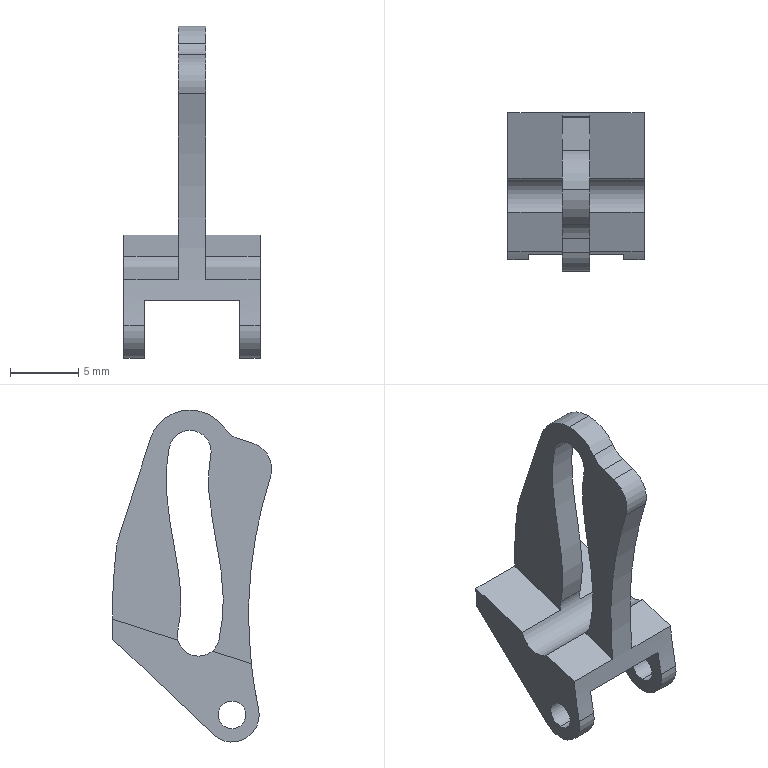Part | SolidWorks | features ICE 2, Extrusion 1, Fillet 1 | 1 solid | 33 faces | box 10 x 11.684 x 24.374 mm | volume 433.075 mm3 | cylinder 16 | plane 15 | spline 2 | commonest cylinder face diameters 4 x5 2.02 x4 3.1 x3 6.1 x2 66 x1 86 x1
STEP:
#1=CARTESIAN_POINT('',(5.,10.718,-6.14));
#2=VERTEX_POINT('',#1);
#3=CARTESIAN_POINT('',(5.,10.718,-8.16));
#4=VERTEX_POINT('',#3);
#5=CARTESIAN_POINT('',(5.,10.718,-7.15));
#6=DIRECTION('',(1.,0.,0.));
#7=DIRECTION('',(0.,0.,-1.));
#8=AXIS2_PLACEMENT_3D('',#5,#6,#7);
#9=CIRCLE('',#8,1.01);
#10=EDGE_CURVE('',#2,#4,#9,.T.);
#11=ORIENTED_EDGE('',*,*,#10,.T.);
#12=CARTESIAN_POINT('',(3.5,10.718,-8.16));
#13=VERTEX_POINT('',#12);
#14=CARTESIAN_POINT('',(1.,10.718,-8.16));
#15=DIRECTION('',(-1.,0.,0.));
#16=VECTOR('',#15,1000.);
#17=LINE('',#14,#16);
#18=EDGE_CURVE('',#4,#13,#17,.T.);
#19=ORIENTED_EDGE('',*,*,#18,.T.);
#20=CARTESIAN_POINT('',(3.5,10.718,-6.14));
#21=VERTEX_POINT('',#20);
#22=CARTESIAN_POINT('',(3.5,10.718,-7.15));
#23=DIRECTION('',(1.,0.,0.));
#24=DIRECTION('',(0.,0.,-1.));
#25=AXIS2_PLACEMENT_3D('',#22,#23,#24);
#26=CIRCLE('',#25,1.01);
#27=EDGE_CURVE('',#21,#13,#26,.T.);
#28=ORIENTED_EDGE('',*,*,#27,.F.);
#29=CARTESIAN_POINT('',(1.,10.718,-6.14));
#30=DIRECTION('',(-1.,0.,0.));
#31=VECTOR('',#30,1000.);
#32=LINE('',#29,#31);
#33=EDGE_CURVE('',#2,#21,#32,.T.);
#34=ORIENTED_EDGE('',*,*,#33,.F.);
#35=EDGE_LOOP('',(#11,#19,#28,#34));
#36=FACE_OUTER_BOUND('',#35,.T.);
#37=CARTESIAN_POINT('',(1.,10.718,-7.15));
#38=DIRECTION('',(-1.,0.,0.));
#39=DIRECTION('',(0.,0.,1.));
#40=AXIS2_PLACEMENT_3D('',#37,#38,#39);
#41=CYLINDRICAL_SURFACE('',#40,1.01);
#42=ADVANCED_FACE('',(#36),#41,.F.);
#43=CARTESIAN_POINT('',(1.,15.317,12.479));
#44=VERTEX_POINT('',#43);
#45=CARTESIAN_POINT('',(1.,13.798,13.724));
#46=VERTEX_POINT('',#45);
#47=CARTESIAN_POINT('',(1.,13.798,12.174));
#48=DIRECTION('',(1.,0.,0.));
#49=DIRECTION('',(0.,0.,-1.));
#50=AXIS2_PLACEMENT_3D('',#47,#48,#49);
#51=CIRCLE('',#50,1.55);
#52=EDGE_CURVE('',#44,#46,#51,.T.);
#53=ORIENTED_EDGE('',*,*,#52,.T.);
#54=CARTESIAN_POINT('',(-1.,13.798,13.724));
#55=VERTEX_POINT('',#54);
#56=CARTESIAN_POINT('',(1.,13.798,13.724));
#57=DIRECTION('',(-1.,0.,0.));
#58=VECTOR('',#57,1000.);
#59=LINE('',#56,#58);
#60=EDGE_CURVE('',#46,#55,#59,.T.);
#61=ORIENTED_EDGE('',*,*,#60,.T.);
#62=CARTESIAN_POINT('',(-1.,15.317,12.479));
#63=VERTEX_POINT('',#62);
#64=CARTESIAN_POINT('',(-1.,13.798,12.174));
#65=DIRECTION('',(1.,0.,0.));
#66=DIRECTION('',(0.,0.,-1.));
#67=AXIS2_PLACEMENT_3D('',#64,#65,#66);
#68=CIRCLE('',#67,1.55);
#69=EDGE_CURVE('',#63,#55,#68,.T.);
#70=ORIENTED_EDGE('',*,*,#69,.F.);
#71=CARTESIAN_POINT('',(1.,15.317,12.479));
#72=DIRECTION('',(-1.,0.,0.));
#73=VECTOR('',#72,1000.);
#74=LINE('',#71,#73);
#75=EDGE_CURVE('',#44,#63,#74,.T.);
#76=ORIENTED_EDGE('',*,*,#75,.F.);
#77=EDGE_LOOP('',(#53,#61,#70,#76));
#78=FACE_OUTER_BOUND('',#77,.T.);
#79=CARTESIAN_POINT('',(1.,13.798,12.174));
#80=DIRECTION('',(-1.,0.,0.));
#81=DIRECTION('',(0.,0.,1.));
#82=AXIS2_PLACEMENT_3D('',#79,#80,#81);
#83=CYLINDRICAL_SURFACE('',#82,1.55);
#84=ADVANCED_FACE('',(#78),#83,.F.);
#85=CARTESIAN_POINT('',(1.,13.798,15.224));
#86=VERTEX_POINT('',#85);
#87=CARTESIAN_POINT('',(1.,11.285,13.903));
#88=VERTEX_POINT('',#87);
#89=CARTESIAN_POINT('',(1.,13.798,12.174));
#90=DIRECTION('',(1.,0.,0.));
#91=DIRECTION('',(0.,0.,-1.));
#92=AXIS2_PLACEMENT_3D('',#89,#90,#91);
#93=CIRCLE('',#92,3.05);
#94=EDGE_CURVE('',#86,#88,#93,.T.);
#95=ORIENTED_EDGE('',*,*,#94,.F.);
#96=CARTESIAN_POINT('',(-1.,13.798,15.224));
#97=VERTEX_POINT('',#96);
#98=CARTESIAN_POINT('',(1.,13.798,15.224));
#99=DIRECTION('',(-1.,0.,0.));
#100=VECTOR('',#99,1000.);
#101=LINE('',#98,#100);
#102=EDGE_CURVE('',#86,#97,#101,.T.);
#103=ORIENTED_EDGE('',*,*,#102,.T.);
#104=CARTESIAN_POINT('',(-1.,11.285,13.903));
#105=VERTEX_POINT('',#104);
#106=CARTESIAN_POINT('',(-1.,13.798,12.174));
#107=DIRECTION('',(1.,0.,0.));
#108=DIRECTION('',(0.,0.,-1.));
#109=AXIS2_PLACEMENT_3D('',#106,#107,#108);
#110=CIRCLE('',#109,3.05);
#111=EDGE_CURVE('',#97,#105,#110,.T.);
#112=ORIENTED_EDGE('',*,*,#111,.T.);
#113=CARTESIAN_POINT('',(1.,11.285,13.903));
#114=DIRECTION('',(1.,0.,0.));
#115=VECTOR('',#114,1000.);
#116=LINE('',#113,#115);
#117=EDGE_CURVE('',#105,#88,#116,.T.);
#118=ORIENTED_EDGE('',*,*,#117,.T.);
#119=EDGE_LOOP('',(#95,#103,#112,#118));
#120=FACE_OUTER_BOUND('',#119,.T.);
#121=CARTESIAN_POINT('',(1.,13.798,12.174));
#122=DIRECTION('',(-1.,0.,0.));
#123=DIRECTION('',(0.,0.,1.));
#124=AXIS2_PLACEMENT_3D('',#121,#122,#123);
#125=CYLINDRICAL_SURFACE('',#124,3.05);
#126=ADVANCED_FACE('',(#120),#125,.T.);
#127=CARTESIAN_POINT('',(-3.5,10.718,-6.14));
#128=VERTEX_POINT('',#127);
#129=CARTESIAN_POINT('',(-3.5,10.718,-8.16));
#130=VERTEX_POINT('',#129);
#131=CARTESIAN_POINT('',(-3.5,10.718,-7.15));
#132=DIRECTION('',(1.,0.,0.));
#133=DIRECTION('',(0.,0.,-1.));
#134=AXIS2_PLACEMENT_3D('',#131,#132,#133);
#135=CIRCLE('',#134,1.01);
#136=EDGE_CURVE('',#128,#130,#135,.T.);
#137=ORIENTED_EDGE('',*,*,#136,.T.);
#138=CARTESIAN_POINT('',(-5.,10.718,-8.16));
#139=VERTEX_POINT('',#138);
#140=CARTESIAN_POINT('',(1.,10.718,-8.16));
#141=DIRECTION('',(-1.,0.,0.));
#142=VECTOR('',#141,1000.);
#143=LINE('',#140,#142);
#144=EDGE_CURVE('',#130,#139,#143,.T.);
#145=ORIENTED_EDGE('',*,*,#144,.T.);
#146=CARTESIAN_POINT('',(-5.,10.718,-6.14));
#147=VERTEX_POINT('',#146);
#148=CARTESIAN_POINT('',(-5.,10.718,-7.15));
#149=DIRECTION('',(1.,0.,0.));
#150=DIRECTION('',(0.,0.,-1.));
#151=AXIS2_PLACEMENT_3D('',#148,#149,#150);
#152=CIRCLE('',#151,1.01);
#153=EDGE_CURVE('',#147,#139,#152,.T.);
#154=ORIENTED_EDGE('',*,*,#153,.F.);
#155=CARTESIAN_POINT('',(1.,10.718,-6.14));
#156=DIRECTION('',(-1.,0.,0.));
#157=VECTOR('',#156,1000.);
#158=LINE('',#155,#157);
#159=EDGE_CURVE('',#128,#147,#158,.T.);
#160=ORIENTED_EDGE('',*,*,#159,.F.);
#161=EDGE_LOOP('',(#137,#145,#154,#160));
#162=FACE_OUTER_BOUND('',#161,.T.);
#163=CARTESIAN_POINT('',(1.,10.718,-7.15));
#164=DIRECTION('',(-1.,0.,0.));
#165=DIRECTION('',(0.,0.,1.));
#166=AXIS2_PLACEMENT_3D('',#163,#164,#165);
#167=CYLINDRICAL_SURFACE('',#166,1.01);
#168=ADVANCED_FACE('',(#162),#167,.F.);
#169=CARTESIAN_POINT('',(-3.5,9.093,-4.942));
#170=VERTEX_POINT('',#169);
#171=CARTESIAN_POINT('',(-3.5,8.762,-6.732));
#172=VERTEX_POINT('',#171);
#173=CARTESIAN_POINT('',(-3.5,-23.51,0.1622));
#174=DIRECTION('',(-1.,0.,0.));
#175=DIRECTION('',(0.,0.,-1.));
#176=AXIS2_PLACEMENT_3D('',#173,#174,#175);
#177=CIRCLE('',#176,33.);
#178=EDGE_CURVE('',#170,#172,#177,.T.);
#179=ORIENTED_EDGE('',*,*,#178,.F.);
#180=CARTESIAN_POINT('',(3.5,9.093,-4.942));
#181=VERTEX_POINT('',#180);
#182=CARTESIAN_POINT('',(-3.5,9.093,-4.942));
#183=DIRECTION('',(1.,0.,0.));
#184=VECTOR('',#183,1000.);
#185=LINE('',#182,#184);
#186=EDGE_CURVE('',#170,#181,#185,.T.);
#187=ORIENTED_EDGE('',*,*,#186,.T.);
#188=CARTESIAN_POINT('',(3.5,8.762,-6.732));
#189=VERTEX_POINT('',#188);
#190=CARTESIAN_POINT('',(3.5,-23.51,0.1622));
#191=DIRECTION('',(-1.,0.,0.));
#192=DIRECTION('',(0.,0.,-1.));
#193=AXIS2_PLACEMENT_3D('',#190,#191,#192);
#194=CIRCLE('',#193,33.);
#195=EDGE_CURVE('',#181,#189,#194,.T.);
#196=ORIENTED_EDGE('',*,*,#195,.T.);
#197=CARTESIAN_POINT('',(5.,8.762,-6.732));
#198=VERTEX_POINT('',#197);
#199=CARTESIAN_POINT('',(1.,8.762,-6.732));
#200=DIRECTION('',(-1.,0.,0.));
#201=VECTOR('',#200,1000.);
#202=LINE('',#199,#201);
#203=EDGE_CURVE('',#198,#189,#202,.T.);
#204=ORIENTED_EDGE('',*,*,#203,.F.);
#205=CARTESIAN_POINT('',(5.,9.297,-3.405));
#206=VERTEX_POINT('',#205);
#207=CARTESIAN_POINT('',(5.,-23.51,0.1622));
#208=DIRECTION('',(-1.,0.,0.));
#209=DIRECTION('',(0.,0.,-1.));
#210=AXIS2_PLACEMENT_3D('',#207,#208,#209);
#211=CIRCLE('',#210,33.);
#212=EDGE_CURVE('',#206,#198,#211,.T.);
#213=ORIENTED_EDGE('',*,*,#212,.F.);
#214=CARTESIAN_POINT('',(1.,9.297,-3.405));
#215=VERTEX_POINT('',#214);
#216=CARTESIAN_POINT('',(5.,9.297,-3.405));
#217=DIRECTION('',(-1.,0.,0.));
#218=VECTOR('',#217,1000.);
#219=LINE('',#216,#218);
#220=EDGE_CURVE('',#206,#215,#219,.T.);
#221=ORIENTED_EDGE('',*,*,#220,.T.);
#222=CARTESIAN_POINT('',(1.,7.902,10.276));
#223=VERTEX_POINT('',#222);
#224=CARTESIAN_POINT('',(1.,-23.51,0.1622));
#225=DIRECTION('',(-1.,0.,0.));
#226=DIRECTION('',(0.,0.,-1.));
#227=AXIS2_PLACEMENT_3D('',#224,#225,#226);
#228=CIRCLE('',#227,33.);
#229=EDGE_CURVE('',#223,#215,#228,.T.);
#230=ORIENTED_EDGE('',*,*,#229,.F.);
#231=CARTESIAN_POINT('',(-1.,7.902,10.276));
#232=VERTEX_POINT('',#231);
#233=CARTESIAN_POINT('',(1.,7.902,10.276));
#234=DIRECTION('',(-1.,0.,0.));
#235=VECTOR('',#234,1000.);
#236=LINE('',#233,#235);
#237=EDGE_CURVE('',#223,#232,#236,.T.);
#238=ORIENTED_EDGE('',*,*,#237,.T.);
#239=CARTESIAN_POINT('',(-1.,9.297,-3.405));
#240=VERTEX_POINT('',#239);
#241=CARTESIAN_POINT('',(-1.,-23.51,0.1622));
#242=DIRECTION('',(-1.,0.,0.));
#243=DIRECTION('',(0.,0.,-1.));
#244=AXIS2_PLACEMENT_3D('',#241,#242,#243);
#245=CIRCLE('',#244,33.);
#246=EDGE_CURVE('',#232,#240,#245,.T.);
#247=ORIENTED_EDGE('',*,*,#246,.T.);
#248=CARTESIAN_POINT('',(-5.,9.297,-3.405));
#249=VERTEX_POINT('',#248);
#250=CARTESIAN_POINT('',(5.,9.297,-3.405));
#251=DIRECTION('',(-1.,0.,0.));
#252=VECTOR('',#251,1000.);
#253=LINE('',#250,#252);
#254=EDGE_CURVE('',#240,#249,#253,.T.);
#255=ORIENTED_EDGE('',*,*,#254,.T.);
#256=CARTESIAN_POINT('',(-5.,8.762,-6.732));
#257=VERTEX_POINT('',#256);
#258=CARTESIAN_POINT('',(-5.,-23.51,0.1622));
#259=DIRECTION('',(-1.,0.,0.));
#260=DIRECTION('',(0.,0.,-1.));
#261=AXIS2_PLACEMENT_3D('',#258,#259,#260);
#262=CIRCLE('',#261,33.);
#263=EDGE_CURVE('',#249,#257,#262,.T.);
#264=ORIENTED_EDGE('',*,*,#263,.T.);
#265=CARTESIAN_POINT('',(1.,8.762,-6.732));
#266=DIRECTION('',(-1.,0.,0.));
#267=VECTOR('',#266,1000.);
#268=LINE('',#265,#267);
#269=EDGE_CURVE('',#172,#257,#268,.T.);
#270=ORIENTED_EDGE('',*,*,#269,.F.);
#271=EDGE_LOOP('',(#179,#187,#196,#204,#213,#221,#230,#238,#247,#255,#264,#270));
#272=FACE_OUTER_BOUND('',#271,.T.);
#273=CARTESIAN_POINT('',(1.,-23.51,0.1622));
#274=DIRECTION('',(-1.,0.,0.));
#275=DIRECTION('',(0.,0.,1.));
#276=AXIS2_PLACEMENT_3D('',#273,#274,#275);
#277=CYLINDRICAL_SURFACE('',#276,33.);
#278=ADVANCED_FACE('',(#272),#277,.F.);
#279=CARTESIAN_POINT('',(-3.5,12.095,-8.6));
#280=VERTEX_POINT('',#279);
#281=CARTESIAN_POINT('',(-3.5,10.718,-7.15));
#282=DIRECTION('',(1.,0.,0.));
#283=DIRECTION('',(0.,0.,-1.));
#284=AXIS2_PLACEMENT_3D('',#281,#282,#283);
#285=CIRCLE('',#284,2.);
#286=EDGE_CURVE('',#172,#280,#285,.T.);
#287=ORIENTED_EDGE('',*,*,#286,.F.);
#288=ORIENTED_EDGE('',*,*,#269,.T.);
#289=CARTESIAN_POINT('',(-5.,12.095,-8.6));
#290=VERTEX_POINT('',#289);
#291=CARTESIAN_POINT('',(-5.,10.718,-7.15));
#292=DIRECTION('',(1.,0.,0.));
#293=DIRECTION('',(0.,0.,-1.));
#294=AXIS2_PLACEMENT_3D('',#291,#292,#293);
#295=CIRCLE('',#294,2.);
#296=EDGE_CURVE('',#257,#290,#295,.T.);
#297=ORIENTED_EDGE('',*,*,#296,.T.);
#298=CARTESIAN_POINT('',(1.,12.095,-8.6));
#299=DIRECTION('',(-1.,0.,0.));
#300=VECTOR('',#299,1000.);
#301=LINE('',#298,#300);
#302=EDGE_CURVE('',#280,#290,#301,.T.);
#303=ORIENTED_EDGE('',*,*,#302,.F.);
#304=EDGE_LOOP('',(#287,#288,#297,#303));
#305=FACE_OUTER_BOUND('',#304,.T.);
#306=CARTESIAN_POINT('',(1.,10.718,-7.15));
#307=DIRECTION('',(-1.,0.,0.));
#308=DIRECTION('',(0.,0.,1.));
#309=AXIS2_PLACEMENT_3D('',#306,#307,#308);
#310=CYLINDRICAL_SURFACE('',#309,2.);
#311=ADVANCED_FACE('',(#305),#310,.T.);
#312=CARTESIAN_POINT('',(-3.5,19.454,-1.606));
#313=VERTEX_POINT('',#312);
#314=CARTESIAN_POINT('',(-3.5,12.095,-8.6));
#315=DIRECTION('',(0.,0.7248,0.6889));
#316=VECTOR('',#315,1000.);
#317=LINE('',#314,#316);
#318=EDGE_CURVE('',#280,#313,#317,.T.);
#319=ORIENTED_EDGE('',*,*,#318,.F.);
#320=ORIENTED_EDGE('',*,*,#302,.T.);
#321=CARTESIAN_POINT('',(-5.,19.454,-1.606));
#322=VERTEX_POINT('',#321);
#323=CARTESIAN_POINT('',(-5.,12.095,-8.6));
#324=DIRECTION('',(0.,0.7248,0.6889));
#325=VECTOR('',#324,1000.);
#326=LINE('',#323,#325);
#327=EDGE_CURVE('',#290,#322,#326,.T.);
#328=ORIENTED_EDGE('',*,*,#327,.T.);
#329=CARTESIAN_POINT('',(1.,19.454,-1.606));
#330=DIRECTION('',(-1.,0.,0.));
#331=VECTOR('',#330,1000.);
#332=LINE('',#329,#331);
#333=EDGE_CURVE('',#313,#322,#332,.T.);
#334=ORIENTED_EDGE('',*,*,#333,.F.);
#335=EDGE_LOOP('',(#319,#320,#328,#334));
#336=FACE_OUTER_BOUND('',#335,.T.);
#337=CARTESIAN_POINT('',(1.,19.454,-1.606));
#338=DIRECTION('',(0.,-0.6889,0.7248));
#339=DIRECTION('',(0.,-0.7248,-0.6889));
#340=AXIS2_PLACEMENT_3D('',#337,#338,#339);
#341=PLANE('',#340);
#342=ADVANCED_FACE('',(#336),#341,.F.);
#343=ORIENTED_EDGE('',*,*,#144,.F.);
#344=CARTESIAN_POINT('',(-3.5,10.718,-7.15));
#345=DIRECTION('',(1.,0.,0.));
#346=DIRECTION('',(0.,0.,-1.));
#347=AXIS2_PLACEMENT_3D('',#344,#345,#346);
#348=CIRCLE('',#347,1.01);
#349=EDGE_CURVE('',#130,#128,#348,.T.);
#350=ORIENTED_EDGE('',*,*,#349,.T.);
#351=ORIENTED_EDGE('',*,*,#159,.T.);
#352=CARTESIAN_POINT('',(-5.,10.718,-7.15));
#353=DIRECTION('',(1.,0.,0.));
#354=DIRECTION('',(0.,0.,-1.));
#355=AXIS2_PLACEMENT_3D('',#352,#353,#354);
#356=CIRCLE('',#355,1.01);
#357=EDGE_CURVE('',#139,#147,#356,.T.);
#358=ORIENTED_EDGE('',*,*,#357,.F.);
#359=EDGE_LOOP('',(#343,#350,#351,#358));
#360=FACE_OUTER_BOUND('',#359,.T.);
#361=CARTESIAN_POINT('',(1.,10.718,-7.15));
#362=DIRECTION('',(-1.,0.,0.));
#363=DIRECTION('',(0.,0.,1.));
#364=AXIS2_PLACEMENT_3D('',#361,#362,#363);
#365=CYLINDRICAL_SURFACE('',#364,1.01);
#366=ADVANCED_FACE('',(#360),#365,.F.);
#367=CARTESIAN_POINT('',(1.,19.489,-0.1238));
#368=VERTEX_POINT('',#367);
#369=CARTESIAN_POINT('',(1.,19.185,5.272));
#370=VERTEX_POINT('',#369);
#371=CARTESIAN_POINT('',(1.,-23.51,0.1622));
#372=DIRECTION('',(1.,0.,0.));
#373=DIRECTION('',(0.,0.,-1.));
#374=AXIS2_PLACEMENT_3D('',#371,#372,#373);
#375=CIRCLE('',#374,43.);
#376=EDGE_CURVE('',#368,#370,#375,.T.);
#377=ORIENTED_EDGE('',*,*,#376,.T.);
#378=CARTESIAN_POINT('',(1.,19.103,5.647));
#379=VERTEX_POINT('',#378);
#380=CARTESIAN_POINT('',(1.,17.199,5.034));
#381=DIRECTION('',(1.,0.,0.));
#382=DIRECTION('',(0.,0.,-1.));
#383=AXIS2_PLACEMENT_3D('',#380,#381,#382);
#384=CIRCLE('',#383,2.);
#385=EDGE_CURVE('',#370,#379,#384,.T.);
#386=ORIENTED_EDGE('',*,*,#385,.T.);
#387=CARTESIAN_POINT('',(1.,16.701,13.109));
#388=VERTEX_POINT('',#387);
#389=CARTESIAN_POINT('',(1.,16.701,13.109));
#390=DIRECTION('',(0.,-0.3065,0.9519));
#391=VECTOR('',#390,1000.);
#392=LINE('',#389,#391);
#393=EDGE_CURVE('',#379,#388,#392,.T.);
#394=ORIENTED_EDGE('',*,*,#393,.T.);
#395=CARTESIAN_POINT('',(1.,13.798,12.174));
#396=DIRECTION('',(1.,0.,0.));
#397=DIRECTION('',(0.,0.,-1.));
#398=AXIS2_PLACEMENT_3D('',#395,#396,#397);
#399=CIRCLE('',#398,3.05);
#400=EDGE_CURVE('',#388,#86,#399,.T.);
#401=ORIENTED_EDGE('',*,*,#400,.T.);
#402=ORIENTED_EDGE('',*,*,#94,.T.);
#403=CARTESIAN_POINT('',(1.,10.25,13.133));
#404=VERTEX_POINT('',#403);
#405=CARTESIAN_POINT('',(1.,9.638,15.037));
#406=DIRECTION('',(-1.,0.,0.));
#407=DIRECTION('',(0.,0.,-1.));
#408=AXIS2_PLACEMENT_3D('',#405,#406,#407);
#409=CIRCLE('',#408,2.);
#410=EDGE_CURVE('',#88,#404,#409,.T.);
#411=ORIENTED_EDGE('',*,*,#410,.T.);
#412=CARTESIAN_POINT('',(1.,9.193,12.792));
#413=VERTEX_POINT('',#412);
#414=CARTESIAN_POINT('',(1.,10.993,13.372));
#415=DIRECTION('',(0.,-0.9519,-0.3065));
#416=VECTOR('',#415,1000.);
#417=LINE('',#414,#416);
#418=EDGE_CURVE('',#404,#413,#417,.T.);
#419=ORIENTED_EDGE('',*,*,#418,.T.);
#420=CARTESIAN_POINT('',(1.,9.806,10.889));
#421=DIRECTION('',(1.,0.,0.));
#422=DIRECTION('',(0.,0.,-1.));
#423=AXIS2_PLACEMENT_3D('',#420,#421,#422);
#424=CIRCLE('',#423,2.);
#425=EDGE_CURVE('',#413,#223,#424,.T.);
#426=ORIENTED_EDGE('',*,*,#425,.T.);
#427=ORIENTED_EDGE('',*,*,#229,.T.);
#428=CARTESIAN_POINT('',(1.,12.177,-2.478));
#429=VERTEX_POINT('',#428);
#430=CARTESIAN_POINT('',(1.,17.92,-0.629));
#431=DIRECTION('',(0.,0.9519,0.3065));
#432=VECTOR('',#431,1000.);
#433=LINE('',#430,#432);
#434=EDGE_CURVE('',#215,#429,#433,.T.);
#435=ORIENTED_EDGE('',*,*,#434,.T.);
#436=CARTESIAN_POINT('',(1.,11.669,-1.652));
#437=VERTEX_POINT('',#436);
#438=CARTESIAN_POINT('',(1.,13.177,-1.294));
#439=DIRECTION('',(1.,0.,0.));
#440=DIRECTION('',(0.,0.,-1.));
#441=AXIS2_PLACEMENT_3D('',#438,#439,#440);
#442=CIRCLE('',#441,1.55);
#443=EDGE_CURVE('',#437,#429,#442,.T.);
#444=ORIENTED_EDGE('',*,*,#443,.F.);
#445=CARTESIAN_POINT('',(1.,12.278,11.869));
#446=VERTEX_POINT('',#445);
#447=CARTESIAN_POINT('',(1.,12.278,11.869));
#448=CARTESIAN_POINT('',(1.,12.472,10.904));
#449=CARTESIAN_POINT('',(1.,12.489,8.974));
#450=CARTESIAN_POINT('',(1.,11.893,5.748));
#451=CARTESIAN_POINT('',(1.,11.376,2.817));
#452=CARTESIAN_POINT('',(1.,11.331,0.3197));
#453=CARTESIAN_POINT('',(1.,11.517,-1.013));
#454=CARTESIAN_POINT('',(1.,11.669,-1.652));
#455=B_SPLINE_CURVE_WITH_KNOTS('',3,(#447,#448,#449,#450,#451,#452,#453,#454),.UNSPECIFIED.,.F.,.F.,(4,1,1,1,1,4),(0.,0.25,0.5,0.75,0.875,1.),.UNSPECIFIED.);
#456=EDGE_CURVE('',#446,#437,#455,.T.);
#457=ORIENTED_EDGE('',*,*,#456,.F.);
#458=CARTESIAN_POINT('',(1.,13.798,12.174));
#459=DIRECTION('',(1.,0.,0.));
#460=DIRECTION('',(0.,0.,-1.));
#461=AXIS2_PLACEMENT_3D('',#458,#459,#460);
#462=CIRCLE('',#461,1.55);
#463=EDGE_CURVE('',#46,#446,#462,.T.);
#464=ORIENTED_EDGE('',*,*,#463,.F.);
#465=ORIENTED_EDGE('',*,*,#52,.F.);
#466=CARTESIAN_POINT('',(1.,14.685,-0.9357));
#467=VERTEX_POINT('',#466);
#468=CARTESIAN_POINT('',(1.,14.685,-0.9357));
#469=CARTESIAN_POINT('',(1.,14.46,0.008806));
#470=CARTESIAN_POINT('',(1.,14.377,1.917));
#471=CARTESIAN_POINT('',(1.,14.829,4.568));
#472=CARTESIAN_POINT('',(1.,15.249,6.836));
#473=CARTESIAN_POINT('',(1.,15.5,8.62));
#474=CARTESIAN_POINT('',(1.,15.57,10.188));
#475=CARTESIAN_POINT('',(1.,15.485,11.482));
#476=CARTESIAN_POINT('',(1.,15.383,12.151));
#477=CARTESIAN_POINT('',(1.,15.317,12.479));
#478=B_SPLINE_CURVE_WITH_KNOTS('',3,(#468,#469,#470,#471,#472,#473,#474,#475,#476,#477),.UNSPECIFIED.,.F.,.F.,(4,1,1,1,1,1,1,4),(0.,0.25,0.5,0.625,0.75,0.875,0.9375,1.),.UNSPECIFIED.);
#479=EDGE_CURVE('',#467,#44,#478,.T.);
#480=ORIENTED_EDGE('',*,*,#479,.F.);
#481=CARTESIAN_POINT('',(1.,14.68,-1.672));
#482=VERTEX_POINT('',#481);
#483=CARTESIAN_POINT('',(1.,13.177,-1.294));
#484=DIRECTION('',(1.,0.,0.));
#485=DIRECTION('',(0.,0.,-1.));
#486=AXIS2_PLACEMENT_3D('',#483,#484,#485);
#487=CIRCLE('',#486,1.55);
#488=EDGE_CURVE('',#482,#467,#487,.T.);
#489=ORIENTED_EDGE('',*,*,#488,.F.);
#490=CARTESIAN_POINT('',(1.,17.92,-0.629));
#491=DIRECTION('',(0.,0.9519,0.3065));
#492=VECTOR('',#491,1000.);
#493=LINE('',#490,#492);
#494=EDGE_CURVE('',#482,#368,#493,.T.);
#495=ORIENTED_EDGE('',*,*,#494,.T.);
#496=EDGE_LOOP('',(#377,#386,#394,#401,#402,#411,#419,#426,#427,#435,#444,#457,#464,#465,#480,#489,#495));
#497=FACE_OUTER_BOUND('',#496,.T.);
#498=CARTESIAN_POINT('',(1.,13.798,12.174));
#499=DIRECTION('',(1.,0.,0.));
#500=DIRECTION('',(0.,0.,-1.));
#501=AXIS2_PLACEMENT_3D('',#498,#499,#500);
#502=PLANE('',#501);
#503=ADVANCED_FACE('',(#497),#502,.T.);
#504=CARTESIAN_POINT('',(-1.,19.103,5.647));
#505=VERTEX_POINT('',#504);
#506=CARTESIAN_POINT('',(-1.,16.701,13.109));
#507=VERTEX_POINT('',#506);
#508=CARTESIAN_POINT('',(-1.,16.701,13.109));
#509=DIRECTION('',(0.,-0.3065,0.9519));
#510=VECTOR('',#509,1000.);
#511=LINE('',#508,#510);
#512=EDGE_CURVE('',#505,#507,#511,.T.);
#513=ORIENTED_EDGE('',*,*,#512,.F.);
#514=CARTESIAN_POINT('',(-1.,19.185,5.272));
#515=VERTEX_POINT('',#514);
#516=CARTESIAN_POINT('',(-1.,17.199,5.034));
#517=DIRECTION('',(-1.,0.,0.));
#518=DIRECTION('',(0.,0.,-1.));
#519=AXIS2_PLACEMENT_3D('',#516,#517,#518);
#520=CIRCLE('',#519,2.);
#521=EDGE_CURVE('',#505,#515,#520,.T.);
#522=ORIENTED_EDGE('',*,*,#521,.T.);
#523=CARTESIAN_POINT('',(-1.,19.489,-0.1238));
#524=VERTEX_POINT('',#523);
#525=CARTESIAN_POINT('',(-1.,-23.51,0.1622));
#526=DIRECTION('',(1.,0.,0.));
#527=DIRECTION('',(0.,0.,-1.));
#528=AXIS2_PLACEMENT_3D('',#525,#526,#527);
#529=CIRCLE('',#528,43.);
#530=EDGE_CURVE('',#524,#515,#529,.T.);
#531=ORIENTED_EDGE('',*,*,#530,.F.);
#532=CARTESIAN_POINT('',(-1.,14.68,-1.672));
#533=VERTEX_POINT('',#532);
#534=CARTESIAN_POINT('',(-1.,17.92,-0.629));
#535=DIRECTION('',(0.,0.9519,0.3065));
#536=VECTOR('',#535,1000.);
#537=LINE('',#534,#536);
#538=EDGE_CURVE('',#533,#524,#537,.T.);
#539=ORIENTED_EDGE('',*,*,#538,.F.);
#540=CARTESIAN_POINT('',(-1.,14.685,-0.9357));
#541=VERTEX_POINT('',#540);
#542=CARTESIAN_POINT('',(-1.,13.177,-1.294));
#543=DIRECTION('',(1.,0.,0.));
#544=DIRECTION('',(0.,0.,-1.));
#545=AXIS2_PLACEMENT_3D('',#542,#543,#544);
#546=CIRCLE('',#545,1.55);
#547=EDGE_CURVE('',#533,#541,#546,.T.);
#548=ORIENTED_EDGE('',*,*,#547,.T.);
#549=CARTESIAN_POINT('',(-1.,14.685,-0.9357));
#550=CARTESIAN_POINT('',(-1.,14.46,0.008806));
#551=CARTESIAN_POINT('',(-1.,14.377,1.917));
#552=CARTESIAN_POINT('',(-1.,14.829,4.568));
#553=CARTESIAN_POINT('',(-1.,15.249,6.836));
#554=CARTESIAN_POINT('',(-1.,15.5,8.62));
#555=CARTESIAN_POINT('',(-1.,15.57,10.188));
#556=CARTESIAN_POINT('',(-1.,15.485,11.482));
#557=CARTESIAN_POINT('',(-1.,15.383,12.151));
#558=CARTESIAN_POINT('',(-1.,15.317,12.479));
#559=B_SPLINE_CURVE_WITH_KNOTS('',3,(#549,#550,#551,#552,#553,#554,#555,#556,#557,#558),.UNSPECIFIED.,.F.,.F.,(4,1,1,1,1,1,1,4),(0.,0.25,0.5,0.625,0.75,0.875,0.9375,1.),.UNSPECIFIED.);
#560=EDGE_CURVE('',#541,#63,#559,.T.);
#561=ORIENTED_EDGE('',*,*,#560,.T.);
#562=ORIENTED_EDGE('',*,*,#69,.T.);
#563=CARTESIAN_POINT('',(-1.,12.278,11.869));
#564=VERTEX_POINT('',#563);
#565=CARTESIAN_POINT('',(-1.,13.798,12.174));
#566=DIRECTION('',(1.,0.,0.));
#567=DIRECTION('',(0.,0.,-1.));
#568=AXIS2_PLACEMENT_3D('',#565,#566,#567);
#569=CIRCLE('',#568,1.55);
#570=EDGE_CURVE('',#55,#564,#569,.T.);
#571=ORIENTED_EDGE('',*,*,#570,.T.);
#572=CARTESIAN_POINT('',(-1.,11.669,-1.652));
#573=VERTEX_POINT('',#572);
#574=CARTESIAN_POINT('',(-1.,12.278,11.869));
#575=CARTESIAN_POINT('',(-1.,12.472,10.904));
#576=CARTESIAN_POINT('',(-1.,12.489,8.974));
#577=CARTESIAN_POINT('',(-1.,11.893,5.748));
#578=CARTESIAN_POINT('',(-1.,11.376,2.817));
#579=CARTESIAN_POINT('',(-1.,11.331,0.3197));
#580=CARTESIAN_POINT('',(-1.,11.517,-1.013));
#581=CARTESIAN_POINT('',(-1.,11.669,-1.652));
#582=B_SPLINE_CURVE_WITH_KNOTS('',3,(#574,#575,#576,#577,#578,#579,#580,#581),.UNSPECIFIED.,.F.,.F.,(4,1,1,1,1,4),(0.,0.25,0.5,0.75,0.875,1.),.UNSPECIFIED.);
#583=EDGE_CURVE('',#564,#573,#582,.T.);
#584=ORIENTED_EDGE('',*,*,#583,.T.);
#585=CARTESIAN_POINT('',(-1.,12.177,-2.478));
#586=VERTEX_POINT('',#585);
#587=CARTESIAN_POINT('',(-1.,13.177,-1.294));
#588=DIRECTION('',(1.,0.,0.));
#589=DIRECTION('',(0.,0.,-1.));
#590=AXIS2_PLACEMENT_3D('',#587,#588,#589);
#591=CIRCLE('',#590,1.55);
#592=EDGE_CURVE('',#573,#586,#591,.T.);
#593=ORIENTED_EDGE('',*,*,#592,.T.);
#594=CARTESIAN_POINT('',(-1.,17.92,-0.629));
#595=DIRECTION('',(0.,0.9519,0.3065));
#596=VECTOR('',#595,1000.);
#597=LINE('',#594,#596);
#598=EDGE_CURVE('',#240,#586,#597,.T.);
#599=ORIENTED_EDGE('',*,*,#598,.F.);
#600=ORIENTED_EDGE('',*,*,#246,.F.);
#601=CARTESIAN_POINT('',(-1.,9.193,12.792));
#602=VERTEX_POINT('',#601);
#603=CARTESIAN_POINT('',(-1.,9.806,10.889));
#604=DIRECTION('',(1.,0.,0.));
#605=DIRECTION('',(0.,0.,-1.));
#606=AXIS2_PLACEMENT_3D('',#603,#604,#605);
#607=CIRCLE('',#606,2.);
#608=EDGE_CURVE('',#602,#232,#607,.T.);
#609=ORIENTED_EDGE('',*,*,#608,.F.);
#610=CARTESIAN_POINT('',(-1.,10.25,13.133));
#611=VERTEX_POINT('',#610);
#612=CARTESIAN_POINT('',(-1.,10.993,13.372));
#613=DIRECTION('',(0.,-0.9519,-0.3065));
#614=VECTOR('',#613,1000.);
#615=LINE('',#612,#614);
#616=EDGE_CURVE('',#611,#602,#615,.T.);
#617=ORIENTED_EDGE('',*,*,#616,.F.);
#618=CARTESIAN_POINT('',(-1.,9.638,15.037));
#619=DIRECTION('',(1.,0.,0.));
#620=DIRECTION('',(0.,0.,-1.));
#621=AXIS2_PLACEMENT_3D('',#618,#619,#620);
#622=CIRCLE('',#621,2.);
#623=EDGE_CURVE('',#611,#105,#622,.T.);
#624=ORIENTED_EDGE('',*,*,#623,.T.);
#625=ORIENTED_EDGE('',*,*,#111,.F.);
#626=CARTESIAN_POINT('',(-1.,13.798,12.174));
#627=DIRECTION('',(1.,0.,0.));
#628=DIRECTION('',(0.,0.,-1.));
#629=AXIS2_PLACEMENT_3D('',#626,#627,#628);
#630=CIRCLE('',#629,3.05);
#631=EDGE_CURVE('',#507,#97,#630,.T.);
#632=ORIENTED_EDGE('',*,*,#631,.F.);
#633=EDGE_LOOP('',(#513,#522,#531,#539,#548,#561,#562,#571,#584,#593,#599,#600,#609,#617,#624,#625,#632));
#634=FACE_OUTER_BOUND('',#633,.T.);
#635=CARTESIAN_POINT('',(-1.,13.798,12.174));
#636=DIRECTION('',(1.,0.,0.));
#637=DIRECTION('',(0.,0.,-1.));
#638=AXIS2_PLACEMENT_3D('',#635,#636,#637);
#639=PLANE('',#638);
#640=ADVANCED_FACE('',(#634),#639,.F.);
#641=ORIENTED_EDGE('',*,*,#102,.F.);
#642=ORIENTED_EDGE('',*,*,#400,.F.);
#643=CARTESIAN_POINT('',(1.,16.701,13.109));
#644=DIRECTION('',(-1.,0.,0.));
#645=VECTOR('',#644,1000.);
#646=LINE('',#643,#645);
#647=EDGE_CURVE('',#388,#507,#646,.T.);
#648=ORIENTED_EDGE('',*,*,#647,.T.);
#649=ORIENTED_EDGE('',*,*,#631,.T.);
#650=EDGE_LOOP('',(#641,#642,#648,#649));
#651=FACE_OUTER_BOUND('',#650,.T.);
#652=CARTESIAN_POINT('',(1.,13.798,12.174));
#653=DIRECTION('',(-1.,0.,0.));
#654=DIRECTION('',(0.,0.,1.));
#655=AXIS2_PLACEMENT_3D('',#652,#653,#654);
#656=CYLINDRICAL_SURFACE('',#655,3.05);
#657=ADVANCED_FACE('',(#651),#656,.T.);
#658=ORIENTED_EDGE('',*,*,#418,.F.);
#659=CARTESIAN_POINT('',(-1.,10.25,13.133));
#660=DIRECTION('',(-1.,0.,0.));
#661=VECTOR('',#660,1000.);
#662=LINE('',#659,#661);
#663=EDGE_CURVE('',#404,#611,#662,.T.);
#664=ORIENTED_EDGE('',*,*,#663,.T.);
#665=ORIENTED_EDGE('',*,*,#616,.T.);
#666=CARTESIAN_POINT('',(1.,9.193,12.792));
#667=DIRECTION('',(-1.,0.,0.));
#668=VECTOR('',#667,1000.);
#669=LINE('',#666,#668);
#670=EDGE_CURVE('',#413,#602,#669,.T.);
#671=ORIENTED_EDGE('',*,*,#670,.F.);
#672=EDGE_LOOP('',(#658,#664,#665,#671));
#673=FACE_OUTER_BOUND('',#672,.T.);
#674=CARTESIAN_POINT('',(1.,10.993,13.372));
#675=DIRECTION('',(0.,0.3065,-0.9519));
#676=DIRECTION('',(0.,0.9519,0.3065));
#677=AXIS2_PLACEMENT_3D('',#674,#675,#676);
#678=PLANE('',#677);
#679=ADVANCED_FACE('',(#673),#678,.F.);
#680=ORIENTED_EDGE('',*,*,#608,.T.);
#681=ORIENTED_EDGE('',*,*,#237,.F.);
#682=ORIENTED_EDGE('',*,*,#425,.F.);
#683=ORIENTED_EDGE('',*,*,#670,.T.);
#684=EDGE_LOOP('',(#680,#681,#682,#683));
#685=FACE_OUTER_BOUND('',#684,.T.);
#686=CARTESIAN_POINT('',(1.,9.806,10.889));
#687=DIRECTION('',(-1.,0.,0.));
#688=DIRECTION('',(0.,0.,1.));
#689=AXIS2_PLACEMENT_3D('',#686,#687,#688);
#690=CYLINDRICAL_SURFACE('',#689,2.);
#691=ADVANCED_FACE('',(#685),#690,.T.);
#692=ORIENTED_EDGE('',*,*,#203,.T.);
#693=CARTESIAN_POINT('',(3.5,12.095,-8.6));
#694=VERTEX_POINT('',#693);
#695=CARTESIAN_POINT('',(3.5,10.718,-7.15));
#696=DIRECTION('',(1.,0.,0.));
#697=DIRECTION('',(0.,0.,-1.));
#698=AXIS2_PLACEMENT_3D('',#695,#696,#697);
#699=CIRCLE('',#698,2.);
#700=EDGE_CURVE('',#189,#694,#699,.T.);
#701=ORIENTED_EDGE('',*,*,#700,.T.);
#702=CARTESIAN_POINT('',(5.,12.095,-8.6));
#703=VERTEX_POINT('',#702);
#704=CARTESIAN_POINT('',(1.,12.095,-8.6));
#705=DIRECTION('',(-1.,0.,0.));
#706=VECTOR('',#705,1000.);
#707=LINE('',#704,#706);
#708=EDGE_CURVE('',#703,#694,#707,.T.);
#709=ORIENTED_EDGE('',*,*,#708,.F.);
#710=CARTESIAN_POINT('',(5.,10.718,-7.15));
#711=DIRECTION('',(1.,0.,0.));
#712=DIRECTION('',(0.,0.,-1.));
#713=AXIS2_PLACEMENT_3D('',#710,#711,#712);
#714=CIRCLE('',#713,2.);
#715=EDGE_CURVE('',#198,#703,#714,.T.);
#716=ORIENTED_EDGE('',*,*,#715,.F.);
#717=EDGE_LOOP('',(#692,#701,#709,#716));
#718=FACE_OUTER_BOUND('',#717,.T.);
#719=CARTESIAN_POINT('',(1.,10.718,-7.15));
#720=DIRECTION('',(-1.,0.,0.));
#721=DIRECTION('',(0.,0.,1.));
#722=AXIS2_PLACEMENT_3D('',#719,#720,#721);
#723=CYLINDRICAL_SURFACE('',#722,2.);
#724=ADVANCED_FACE('',(#718),#723,.T.);
#725=ORIENTED_EDGE('',*,*,#708,.T.);
#726=CARTESIAN_POINT('',(3.5,19.454,-1.606));
#727=VERTEX_POINT('',#726);
#728=CARTESIAN_POINT('',(3.5,12.095,-8.6));
#729=DIRECTION('',(0.,0.7248,0.6889));
#730=VECTOR('',#729,1000.);
#731=LINE('',#728,#730);
#732=EDGE_CURVE('',#694,#727,#731,.T.);
#733=ORIENTED_EDGE('',*,*,#732,.T.);
#734=CARTESIAN_POINT('',(5.,19.454,-1.606));
#735=VERTEX_POINT('',#734);
#736=CARTESIAN_POINT('',(1.,19.454,-1.606));
#737=DIRECTION('',(-1.,0.,0.));
#738=VECTOR('',#737,1000.);
#739=LINE('',#736,#738);
#740=EDGE_CURVE('',#735,#727,#739,.T.);
#741=ORIENTED_EDGE('',*,*,#740,.F.);
#742=CARTESIAN_POINT('',(5.,12.095,-8.6));
#743=DIRECTION('',(0.,0.7248,0.6889));
#744=VECTOR('',#743,1000.);
#745=LINE('',#742,#744);
#746=EDGE_CURVE('',#703,#735,#745,.T.);
#747=ORIENTED_EDGE('',*,*,#746,.F.);
#748=EDGE_LOOP('',(#725,#733,#741,#747));
#749=FACE_OUTER_BOUND('',#748,.T.);
#750=CARTESIAN_POINT('',(1.,19.454,-1.606));
#751=DIRECTION('',(0.,-0.6889,0.7248));
#752=DIRECTION('',(0.,-0.7248,-0.6889));
#753=AXIS2_PLACEMENT_3D('',#750,#751,#752);
#754=PLANE('',#753);
#755=ADVANCED_FACE('',(#749),#754,.F.);
#756=ORIENTED_EDGE('',*,*,#530,.T.);
#757=CARTESIAN_POINT('',(1.,19.185,5.272));
#758=DIRECTION('',(1.,0.,0.));
#759=VECTOR('',#758,1000.);
#760=LINE('',#757,#759);
#761=EDGE_CURVE('',#515,#370,#760,.T.);
#762=ORIENTED_EDGE('',*,*,#761,.T.);
#763=ORIENTED_EDGE('',*,*,#376,.F.);
#764=CARTESIAN_POINT('',(5.,19.489,-0.1238));
#765=VERTEX_POINT('',#764);
#766=CARTESIAN_POINT('',(5.,19.489,-0.1238));
#767=DIRECTION('',(-1.,0.,0.));
#768=VECTOR('',#767,1000.);
#769=LINE('',#766,#768);
#770=EDGE_CURVE('',#765,#368,#769,.T.);
#771=ORIENTED_EDGE('',*,*,#770,.F.);
#772=CARTESIAN_POINT('',(5.,-23.51,0.1622));
#773=DIRECTION('',(1.,0.,0.));
#774=DIRECTION('',(0.,0.,-1.));
#775=AXIS2_PLACEMENT_3D('',#772,#773,#774);
#776=CIRCLE('',#775,43.);
#777=EDGE_CURVE('',#735,#765,#776,.T.);
#778=ORIENTED_EDGE('',*,*,#777,.F.);
#779=ORIENTED_EDGE('',*,*,#740,.T.);
#780=CARTESIAN_POINT('',(-3.5,19.454,-1.606));
#781=DIRECTION('',(1.,0.,0.));
#782=VECTOR('',#781,1000.);
#783=LINE('',#780,#782);
#784=EDGE_CURVE('',#313,#727,#783,.T.);
#785=ORIENTED_EDGE('',*,*,#784,.F.);
#786=ORIENTED_EDGE('',*,*,#333,.T.);
#787=CARTESIAN_POINT('',(-5.,19.489,-0.1238));
#788=VERTEX_POINT('',#787);
#789=CARTESIAN_POINT('',(-5.,-23.51,0.1622));
#790=DIRECTION('',(1.,0.,0.));
#791=DIRECTION('',(0.,0.,-1.));
#792=AXIS2_PLACEMENT_3D('',#789,#790,#791);
#793=CIRCLE('',#792,43.);
#794=EDGE_CURVE('',#322,#788,#793,.T.);
#795=ORIENTED_EDGE('',*,*,#794,.T.);
#796=CARTESIAN_POINT('',(5.,19.489,-0.1238));
#797=DIRECTION('',(-1.,0.,0.));
#798=VECTOR('',#797,1000.);
#799=LINE('',#796,#798);
#800=EDGE_CURVE('',#524,#788,#799,.T.);
#801=ORIENTED_EDGE('',*,*,#800,.F.);
#802=EDGE_LOOP('',(#756,#762,#763,#771,#778,#779,#785,#786,#795,#801));
#803=FACE_OUTER_BOUND('',#802,.T.);
#804=CARTESIAN_POINT('',(1.,-23.51,0.1622));
#805=DIRECTION('',(-1.,0.,0.));
#806=DIRECTION('',(0.,0.,1.));
#807=AXIS2_PLACEMENT_3D('',#804,#805,#806);
#808=CYLINDRICAL_SURFACE('',#807,43.);
#809=ADVANCED_FACE('',(#803),#808,.T.);
#810=ORIENTED_EDGE('',*,*,#393,.F.);
#811=CARTESIAN_POINT('',(1.,19.103,5.647));
#812=DIRECTION('',(-1.,0.,0.));
#813=VECTOR('',#812,1000.);
#814=LINE('',#811,#813);
#815=EDGE_CURVE('',#379,#505,#814,.T.);
#816=ORIENTED_EDGE('',*,*,#815,.T.);
#817=ORIENTED_EDGE('',*,*,#512,.T.);
#818=ORIENTED_EDGE('',*,*,#647,.F.);
#819=EDGE_LOOP('',(#810,#816,#817,#818));
#820=FACE_OUTER_BOUND('',#819,.T.);
#821=CARTESIAN_POINT('',(1.,16.701,13.109));
#822=DIRECTION('',(0.,-0.9519,-0.3065));
#823=DIRECTION('',(0.,0.3065,-0.9519));
#824=AXIS2_PLACEMENT_3D('',#821,#822,#823);
#825=PLANE('',#824);
#826=ADVANCED_FACE('',(#820),#825,.F.);
#827=ORIENTED_EDGE('',*,*,#560,.F.);
#828=CARTESIAN_POINT('',(1.,14.685,-0.9357));
#829=DIRECTION('',(-1.,0.,0.));
#830=VECTOR('',#829,1000.);
#831=LINE('',#828,#830);
#832=EDGE_CURVE('',#467,#541,#831,.T.);
#833=ORIENTED_EDGE('',*,*,#832,.F.);
#834=ORIENTED_EDGE('',*,*,#479,.T.);
#835=ORIENTED_EDGE('',*,*,#75,.T.);
#836=EDGE_LOOP('',(#827,#833,#834,#835));
#837=FACE_OUTER_BOUND('',#836,.T.);
#838=CARTESIAN_POINT('',(1.,14.685,-0.9357));
#839=CARTESIAN_POINT('',(-1.,14.685,-0.9357));
#840=CARTESIAN_POINT('',(1.,14.46,0.008806));
#841=CARTESIAN_POINT('',(-1.,14.46,0.008806));
#842=CARTESIAN_POINT('',(1.,14.377,1.917));
#843=CARTESIAN_POINT('',(-1.,14.377,1.917));
#844=CARTESIAN_POINT('',(1.,14.829,4.568));
#845=CARTESIAN_POINT('',(-1.,14.829,4.568));
#846=CARTESIAN_POINT('',(1.,15.249,6.836));
#847=CARTESIAN_POINT('',(-1.,15.249,6.836));
#848=CARTESIAN_POINT('',(1.,15.5,8.62));
#849=CARTESIAN_POINT('',(-1.,15.5,8.62));
#850=CARTESIAN_POINT('',(1.,15.57,10.188));
#851=CARTESIAN_POINT('',(-1.,15.57,10.188));
#852=CARTESIAN_POINT('',(1.,15.485,11.482));
#853=CARTESIAN_POINT('',(-1.,15.485,11.482));
#854=CARTESIAN_POINT('',(1.,15.383,12.151));
#855=CARTESIAN_POINT('',(-1.,15.383,12.151));
#856=CARTESIAN_POINT('',(1.,15.317,12.479));
#857=CARTESIAN_POINT('',(-1.,15.317,12.479));
#858=B_SPLINE_SURFACE_WITH_KNOTS('',3,1,((#838,#839),(#840,#841),(#842,#843),(#844,#845),(#846,#847),(#848,#849),(#850,#851),(#852,#853),(#854,#855),(#856,#857)),.UNSPECIFIED.,.F.,.F.,.F.,(4,1,1,1,1,1,1,4),(2,2),(0.,0.25,0.5,0.625,0.75,0.875,0.9375,1.),(0.,1.),.UNSPECIFIED.);
#859=ADVANCED_FACE('',(#837),#858,.T.);
#860=ORIENTED_EDGE('',*,*,#60,.F.);
#861=ORIENTED_EDGE('',*,*,#463,.T.);
#862=CARTESIAN_POINT('',(1.,12.278,11.869));
#863=DIRECTION('',(-1.,0.,0.));
#864=VECTOR('',#863,1000.);
#865=LINE('',#862,#864);
#866=EDGE_CURVE('',#446,#564,#865,.T.);
#867=ORIENTED_EDGE('',*,*,#866,.T.);
#868=ORIENTED_EDGE('',*,*,#570,.F.);
#869=EDGE_LOOP('',(#860,#861,#867,#868));
#870=FACE_OUTER_BOUND('',#869,.T.);
#871=CARTESIAN_POINT('',(1.,13.798,12.174));
#872=DIRECTION('',(-1.,0.,0.));
#873=DIRECTION('',(0.,0.,1.));
#874=AXIS2_PLACEMENT_3D('',#871,#872,#873);
#875=CYLINDRICAL_SURFACE('',#874,1.55);
#876=ADVANCED_FACE('',(#870),#875,.F.);
#877=ORIENTED_EDGE('',*,*,#583,.F.);
#878=ORIENTED_EDGE('',*,*,#866,.F.);
#879=ORIENTED_EDGE('',*,*,#456,.T.);
#880=CARTESIAN_POINT('',(1.,11.669,-1.652));
#881=DIRECTION('',(-1.,0.,0.));
#882=VECTOR('',#881,1000.);
#883=LINE('',#880,#882);
#884=EDGE_CURVE('',#437,#573,#883,.T.);
#885=ORIENTED_EDGE('',*,*,#884,.T.);
#886=EDGE_LOOP('',(#877,#878,#879,#885));
#887=FACE_OUTER_BOUND('',#886,.T.);
#888=CARTESIAN_POINT('',(1.,12.278,11.869));
#889=CARTESIAN_POINT('',(-1.,12.278,11.869));
#890=CARTESIAN_POINT('',(1.,12.472,10.904));
#891=CARTESIAN_POINT('',(-1.,12.472,10.904));
#892=CARTESIAN_POINT('',(1.,12.489,8.974));
#893=CARTESIAN_POINT('',(-1.,12.489,8.974));
#894=CARTESIAN_POINT('',(1.,11.893,5.748));
#895=CARTESIAN_POINT('',(-1.,11.893,5.748));
#896=CARTESIAN_POINT('',(1.,11.376,2.817));
#897=CARTESIAN_POINT('',(-1.,11.376,2.817));
#898=CARTESIAN_POINT('',(1.,11.331,0.3197));
#899=CARTESIAN_POINT('',(-1.,11.331,0.3197));
#900=CARTESIAN_POINT('',(1.,11.517,-1.013));
#901=CARTESIAN_POINT('',(-1.,11.517,-1.013));
#902=CARTESIAN_POINT('',(1.,11.669,-1.652));
#903=CARTESIAN_POINT('',(-1.,11.669,-1.652));
#904=B_SPLINE_SURFACE_WITH_KNOTS('',3,1,((#888,#889),(#890,#891),(#892,#893),(#894,#895),(#896,#897),(#898,#899),(#900,#901),(#902,#903)),.UNSPECIFIED.,.F.,.F.,.F.,(4,1,1,1,1,4),(2,2),(0.,0.25,0.5,0.75,0.875,1.),(0.,1.),.UNSPECIFIED.);
#905=ADVANCED_FACE('',(#887),#904,.T.);
#906=ORIENTED_EDGE('',*,*,#443,.T.);
#907=CARTESIAN_POINT('',(5.,12.177,-2.478));
#908=VERTEX_POINT('',#907);
#909=CARTESIAN_POINT('',(5.,12.177,-2.478));
#910=DIRECTION('',(-1.,0.,0.));
#911=VECTOR('',#910,1000.);
#912=LINE('',#909,#911);
#913=EDGE_CURVE('',#908,#429,#912,.T.);
#914=ORIENTED_EDGE('',*,*,#913,.F.);
#915=CARTESIAN_POINT('',(5.,14.68,-1.672));
#916=VERTEX_POINT('',#915);
#917=CARTESIAN_POINT('',(5.,13.177,-1.294));
#918=DIRECTION('',(-1.,0.,0.));
#919=DIRECTION('',(0.,0.,-1.));
#920=AXIS2_PLACEMENT_3D('',#917,#918,#919);
#921=CIRCLE('',#920,1.55);
#922=EDGE_CURVE('',#916,#908,#921,.T.);
#923=ORIENTED_EDGE('',*,*,#922,.F.);
#924=CARTESIAN_POINT('',(5.,14.68,-1.672));
#925=DIRECTION('',(-1.,0.,0.));
#926=VECTOR('',#925,1000.);
#927=LINE('',#924,#926);
#928=EDGE_CURVE('',#916,#482,#927,.T.);
#929=ORIENTED_EDGE('',*,*,#928,.T.);
#930=ORIENTED_EDGE('',*,*,#488,.T.);
#931=ORIENTED_EDGE('',*,*,#832,.T.);
#932=ORIENTED_EDGE('',*,*,#547,.F.);
#933=CARTESIAN_POINT('',(-5.,14.68,-1.672));
#934=VERTEX_POINT('',#933);
#935=CARTESIAN_POINT('',(5.,14.68,-1.672));
#936=DIRECTION('',(-1.,0.,0.));
#937=VECTOR('',#936,1000.);
#938=LINE('',#935,#937);
#939=EDGE_CURVE('',#533,#934,#938,.T.);
#940=ORIENTED_EDGE('',*,*,#939,.T.);
#941=CARTESIAN_POINT('',(-5.,12.177,-2.478));
#942=VERTEX_POINT('',#941);
#943=CARTESIAN_POINT('',(-5.,13.177,-1.294));
#944=DIRECTION('',(-1.,0.,0.));
#945=DIRECTION('',(0.,0.,-1.));
#946=AXIS2_PLACEMENT_3D('',#943,#944,#945);
#947=CIRCLE('',#946,1.55);
#948=EDGE_CURVE('',#934,#942,#947,.T.);
#949=ORIENTED_EDGE('',*,*,#948,.T.);
#950=CARTESIAN_POINT('',(5.,12.177,-2.478));
#951=DIRECTION('',(-1.,0.,0.));
#952=VECTOR('',#951,1000.);
#953=LINE('',#950,#952);
#954=EDGE_CURVE('',#586,#942,#953,.T.);
#955=ORIENTED_EDGE('',*,*,#954,.F.);
#956=ORIENTED_EDGE('',*,*,#592,.F.);
#957=ORIENTED_EDGE('',*,*,#884,.F.);
#958=EDGE_LOOP('',(#906,#914,#923,#929,#930,#931,#932,#940,#949,#955,#956,#957));
#959=FACE_OUTER_BOUND('',#958,.T.);
#960=CARTESIAN_POINT('',(1.,13.177,-1.294));
#961=DIRECTION('',(-1.,0.,0.));
#962=DIRECTION('',(0.,0.,1.));
#963=AXIS2_PLACEMENT_3D('',#960,#961,#962);
#964=CYLINDRICAL_SURFACE('',#963,1.55);
#965=ADVANCED_FACE('',(#959),#964,.F.);
#966=ORIENTED_EDGE('',*,*,#254,.F.);
#967=ORIENTED_EDGE('',*,*,#598,.T.);
#968=ORIENTED_EDGE('',*,*,#954,.T.);
#969=CARTESIAN_POINT('',(-5.,12.177,-2.478));
#970=DIRECTION('',(0.,-0.9519,-0.3065));
#971=VECTOR('',#970,1000.);
#972=LINE('',#969,#971);
#973=EDGE_CURVE('',#942,#249,#972,.T.);
#974=ORIENTED_EDGE('',*,*,#973,.T.);
#975=EDGE_LOOP('',(#966,#967,#968,#974));
#976=FACE_OUTER_BOUND('',#975,.T.);
#977=CARTESIAN_POINT('',(5.,12.177,-2.478));
#978=DIRECTION('',(0.,0.3065,-0.9519));
#979=DIRECTION('',(0.,0.9519,0.3065));
#980=AXIS2_PLACEMENT_3D('',#977,#978,#979);
#981=PLANE('',#980);
#982=ADVANCED_FACE('',(#976),#981,.F.);
#983=ORIENTED_EDGE('',*,*,#939,.F.);
#984=ORIENTED_EDGE('',*,*,#538,.T.);
#985=ORIENTED_EDGE('',*,*,#800,.T.);
#986=CARTESIAN_POINT('',(-5.,19.489,-0.1238));
#987=DIRECTION('',(0.,-0.9519,-0.3065));
#988=VECTOR('',#987,1000.);
#989=LINE('',#986,#988);
#990=EDGE_CURVE('',#788,#934,#989,.T.);
#991=ORIENTED_EDGE('',*,*,#990,.T.);
#992=EDGE_LOOP('',(#983,#984,#985,#991));
#993=FACE_OUTER_BOUND('',#992,.T.);
#994=CARTESIAN_POINT('',(5.,19.489,-0.1238));
#995=DIRECTION('',(0.,0.3065,-0.9519));
#996=DIRECTION('',(0.,0.9519,0.3065));
#997=AXIS2_PLACEMENT_3D('',#994,#995,#996);
#998=PLANE('',#997);
#999=ADVANCED_FACE('',(#993),#998,.F.);
#1000=ORIENTED_EDGE('',*,*,#794,.F.);
#1001=ORIENTED_EDGE('',*,*,#327,.F.);
#1002=ORIENTED_EDGE('',*,*,#296,.F.);
#1003=ORIENTED_EDGE('',*,*,#263,.F.);
#1004=ORIENTED_EDGE('',*,*,#973,.F.);
#1005=ORIENTED_EDGE('',*,*,#948,.F.);
#1006=ORIENTED_EDGE('',*,*,#990,.F.);
#1007=EDGE_LOOP('',(#1000,#1001,#1002,#1003,#1004,#1005,#1006));
#1008=FACE_OUTER_BOUND('',#1007,.T.);
#1009=ORIENTED_EDGE('',*,*,#153,.T.);
#1010=ORIENTED_EDGE('',*,*,#357,.T.);
#1011=EDGE_LOOP('',(#1009,#1010));
#1012=FACE_BOUND('',#1011,.T.);
#1013=CARTESIAN_POINT('',(-5.,-23.51,0.1622));
#1014=DIRECTION('',(1.,0.,0.));
#1015=DIRECTION('',(0.,0.,-1.));
#1016=AXIS2_PLACEMENT_3D('',#1013,#1014,#1015);
#1017=PLANE('',#1016);
#1018=ADVANCED_FACE('',(#1008,#1012),#1017,.F.);
#1019=ORIENTED_EDGE('',*,*,#18,.F.);
#1020=CARTESIAN_POINT('',(5.,10.718,-7.15));
#1021=DIRECTION('',(1.,0.,0.));
#1022=DIRECTION('',(0.,0.,-1.));
#1023=AXIS2_PLACEMENT_3D('',#1020,#1021,#1022);
#1024=CIRCLE('',#1023,1.01);
#1025=EDGE_CURVE('',#4,#2,#1024,.T.);
#1026=ORIENTED_EDGE('',*,*,#1025,.T.);
#1027=ORIENTED_EDGE('',*,*,#33,.T.);
#1028=CARTESIAN_POINT('',(3.5,10.718,-7.15));
#1029=DIRECTION('',(1.,0.,0.));
#1030=DIRECTION('',(0.,0.,-1.));
#1031=AXIS2_PLACEMENT_3D('',#1028,#1029,#1030);
#1032=CIRCLE('',#1031,1.01);
#1033=EDGE_CURVE('',#13,#21,#1032,.T.);
#1034=ORIENTED_EDGE('',*,*,#1033,.F.);
#1035=EDGE_LOOP('',(#1019,#1026,#1027,#1034));
#1036=FACE_OUTER_BOUND('',#1035,.T.);
#1037=CARTESIAN_POINT('',(1.,10.718,-7.15));
#1038=DIRECTION('',(-1.,0.,0.));
#1039=DIRECTION('',(0.,0.,1.));
#1040=AXIS2_PLACEMENT_3D('',#1037,#1038,#1039);
#1041=CYLINDRICAL_SURFACE('',#1040,1.01);
#1042=ADVANCED_FACE('',(#1036),#1041,.F.);
#1043=ORIENTED_EDGE('',*,*,#777,.T.);
#1044=CARTESIAN_POINT('',(5.,19.489,-0.1238));
#1045=DIRECTION('',(0.,-0.9519,-0.3065));
#1046=VECTOR('',#1045,1000.);
#1047=LINE('',#1044,#1046);
#1048=EDGE_CURVE('',#765,#916,#1047,.T.);
#1049=ORIENTED_EDGE('',*,*,#1048,.T.);
#1050=ORIENTED_EDGE('',*,*,#922,.T.);
#1051=CARTESIAN_POINT('',(5.,12.177,-2.478));
#1052=DIRECTION('',(0.,-0.9519,-0.3065));
#1053=VECTOR('',#1052,1000.);
#1054=LINE('',#1051,#1053);
#1055=EDGE_CURVE('',#908,#206,#1054,.T.);
#1056=ORIENTED_EDGE('',*,*,#1055,.T.);
#1057=ORIENTED_EDGE('',*,*,#212,.T.);
#1058=ORIENTED_EDGE('',*,*,#715,.T.);
#1059=ORIENTED_EDGE('',*,*,#746,.T.);
#1060=EDGE_LOOP('',(#1043,#1049,#1050,#1056,#1057,#1058,#1059));
#1061=FACE_OUTER_BOUND('',#1060,.T.);
#1062=ORIENTED_EDGE('',*,*,#10,.F.);
#1063=ORIENTED_EDGE('',*,*,#1025,.F.);
#1064=EDGE_LOOP('',(#1062,#1063));
#1065=FACE_BOUND('',#1064,.T.);
#1066=CARTESIAN_POINT('',(5.,-23.51,0.1622));
#1067=DIRECTION('',(1.,0.,0.));
#1068=DIRECTION('',(0.,0.,-1.));
#1069=AXIS2_PLACEMENT_3D('',#1066,#1067,#1068);
#1070=PLANE('',#1069);
#1071=ADVANCED_FACE('',(#1061,#1065),#1070,.T.);
#1072=ORIENTED_EDGE('',*,*,#494,.F.);
#1073=ORIENTED_EDGE('',*,*,#928,.F.);
#1074=ORIENTED_EDGE('',*,*,#1048,.F.);
#1075=ORIENTED_EDGE('',*,*,#770,.T.);
#1076=EDGE_LOOP('',(#1072,#1073,#1074,#1075));
#1077=FACE_OUTER_BOUND('',#1076,.T.);
#1078=CARTESIAN_POINT('',(5.,19.489,-0.1238));
#1079=DIRECTION('',(0.,0.3065,-0.9519));
#1080=DIRECTION('',(0.,0.9519,0.3065));
#1081=AXIS2_PLACEMENT_3D('',#1078,#1079,#1080);
#1082=PLANE('',#1081);
#1083=ADVANCED_FACE('',(#1077),#1082,.F.);
#1084=ORIENTED_EDGE('',*,*,#434,.F.);
#1085=ORIENTED_EDGE('',*,*,#220,.F.);
#1086=ORIENTED_EDGE('',*,*,#1055,.F.);
#1087=ORIENTED_EDGE('',*,*,#913,.T.);
#1088=EDGE_LOOP('',(#1084,#1085,#1086,#1087));
#1089=FACE_OUTER_BOUND('',#1088,.T.);
#1090=CARTESIAN_POINT('',(5.,12.177,-2.478));
#1091=DIRECTION('',(0.,0.3065,-0.9519));
#1092=DIRECTION('',(0.,0.9519,0.3065));
#1093=AXIS2_PLACEMENT_3D('',#1090,#1091,#1092);
#1094=PLANE('',#1093);
#1095=ADVANCED_FACE('',(#1089),#1094,.F.);
#1096=CARTESIAN_POINT('',(3.5,19.454,-1.606));
#1097=DIRECTION('',(0.,-0.9519,-0.3065));
#1098=VECTOR('',#1097,1000.);
#1099=LINE('',#1096,#1098);
#1100=EDGE_CURVE('',#727,#181,#1099,.T.);
#1101=ORIENTED_EDGE('',*,*,#1100,.T.);
#1102=ORIENTED_EDGE('',*,*,#186,.F.);
#1103=CARTESIAN_POINT('',(-3.5,19.454,-1.606));
#1104=DIRECTION('',(0.,-0.9519,-0.3065));
#1105=VECTOR('',#1104,1000.);
#1106=LINE('',#1103,#1105);
#1107=EDGE_CURVE('',#313,#170,#1106,.T.);
#1108=ORIENTED_EDGE('',*,*,#1107,.F.);
#1109=ORIENTED_EDGE('',*,*,#784,.T.);
#1110=EDGE_LOOP('',(#1101,#1102,#1108,#1109));
#1111=FACE_OUTER_BOUND('',#1110,.T.);
#1112=CARTESIAN_POINT('',(-3.5,19.454,-1.606));
#1113=DIRECTION('',(0.,-0.3065,0.9519));
#1114=DIRECTION('',(0.,-0.9519,-0.3065));
#1115=AXIS2_PLACEMENT_3D('',#1112,#1113,#1114);
#1116=PLANE('',#1115);
#1117=ADVANCED_FACE('',(#1111),#1116,.F.);
#1118=ORIENTED_EDGE('',*,*,#136,.F.);
#1119=ORIENTED_EDGE('',*,*,#349,.F.);
#1120=EDGE_LOOP('',(#1118,#1119));
#1121=FACE_BOUND('',#1120,.T.);
#1122=ORIENTED_EDGE('',*,*,#178,.T.);
#1123=ORIENTED_EDGE('',*,*,#286,.T.);
#1124=ORIENTED_EDGE('',*,*,#318,.T.);
#1125=ORIENTED_EDGE('',*,*,#1107,.T.);
#1126=EDGE_LOOP('',(#1122,#1123,#1124,#1125));
#1127=FACE_OUTER_BOUND('',#1126,.T.);
#1128=CARTESIAN_POINT('',(-3.5,-23.51,0.1622));
#1129=DIRECTION('',(1.,0.,0.));
#1130=DIRECTION('',(0.,0.,-1.));
#1131=AXIS2_PLACEMENT_3D('',#1128,#1129,#1130);
#1132=PLANE('',#1131);
#1133=ADVANCED_FACE('',(#1121,#1127),#1132,.T.);
#1134=ORIENTED_EDGE('',*,*,#27,.T.);
#1135=ORIENTED_EDGE('',*,*,#1033,.T.);
#1136=EDGE_LOOP('',(#1134,#1135));
#1137=FACE_BOUND('',#1136,.T.);
#1138=ORIENTED_EDGE('',*,*,#195,.F.);
#1139=ORIENTED_EDGE('',*,*,#1100,.F.);
#1140=ORIENTED_EDGE('',*,*,#732,.F.);
#1141=ORIENTED_EDGE('',*,*,#700,.F.);
#1142=EDGE_LOOP('',(#1138,#1139,#1140,#1141));
#1143=FACE_OUTER_BOUND('',#1142,.T.);
#1144=CARTESIAN_POINT('',(3.5,-23.51,0.1622));
#1145=DIRECTION('',(1.,0.,0.));
#1146=DIRECTION('',(0.,0.,-1.));
#1147=AXIS2_PLACEMENT_3D('',#1144,#1145,#1146);
#1148=PLANE('',#1147);
#1149=ADVANCED_FACE('',(#1137,#1143),#1148,.F.);
#1150=ORIENTED_EDGE('',*,*,#385,.F.);
#1151=ORIENTED_EDGE('',*,*,#761,.F.);
#1152=ORIENTED_EDGE('',*,*,#521,.F.);
#1153=ORIENTED_EDGE('',*,*,#815,.F.);
#1154=EDGE_LOOP('',(#1150,#1151,#1152,#1153));
#1155=FACE_OUTER_BOUND('',#1154,.T.);
#1156=CARTESIAN_POINT('',(1.,17.199,5.034));
#1157=DIRECTION('',(-1.,0.,0.));
#1158=DIRECTION('',(0.,0.,1.));
#1159=AXIS2_PLACEMENT_3D('',#1156,#1157,#1158);
#1160=CYLINDRICAL_SURFACE('',#1159,2.);
#1161=ADVANCED_FACE('',(#1155),#1160,.T.);
#1162=ORIENTED_EDGE('',*,*,#410,.F.);
#1163=ORIENTED_EDGE('',*,*,#117,.F.);
#1164=ORIENTED_EDGE('',*,*,#623,.F.);
#1165=ORIENTED_EDGE('',*,*,#663,.F.);
#1166=EDGE_LOOP('',(#1162,#1163,#1164,#1165));
#1167=FACE_OUTER_BOUND('',#1166,.T.);
#1168=CARTESIAN_POINT('',(1.,9.638,15.037));
#1169=DIRECTION('',(-1.,0.,0.));
#1170=DIRECTION('',(0.,0.,1.));
#1171=AXIS2_PLACEMENT_3D('',#1168,#1169,#1170);
#1172=CYLINDRICAL_SURFACE('',#1171,2.);
#1173=ADVANCED_FACE('',(#1167),#1172,.F.);
#1174=CLOSED_SHELL('',(#42,#84,#126,#168,#278,#311,#342,#366,#503,#640,#657,#679,#691,#724,#755,#809,#826,#859,#876,#905,#965,#982,#999,#1018,#1042,#1071,#1083,#1095,#1117,#1133,#1149,#1161,#1173));
#1175=MANIFOLD_SOLID_BREP('',#1174);
#1176=CARTESIAN_POINT('',(0.,0.,0.));
#1177=DIRECTION('',(0.,0.,1.));
#1178=DIRECTION('',(1.,0.,0.));
#1179=AXIS2_PLACEMENT_3D('',#1176,#1177,#1178);
#1180=(LENGTH_UNIT()NAMED_UNIT(*)SI_UNIT(.MILLI.,.METRE.));
#1181=UNCERTAINTY_MEASURE_WITH_UNIT(LENGTH_MEASURE(0.00001),#1180,'','');
#1182=(NAMED_UNIT(*)PLANE_ANGLE_UNIT()SI_UNIT($,.RADIAN.));
#1183=(NAMED_UNIT(*)SI_UNIT($,.STERADIAN.)SOLID_ANGLE_UNIT());
#1184=(GEOMETRIC_REPRESENTATION_CONTEXT(3)GLOBAL_UNCERTAINTY_ASSIGNED_CONTEXT((#1181))GLOBAL_UNIT_ASSIGNED_CONTEXT((#1180,#1182,#1183))REPRESENTATION_CONTEXT('',''));
#1185=ADVANCED_BREP_SHAPE_REPRESENTATION('',(#1175,#1179),#1184);